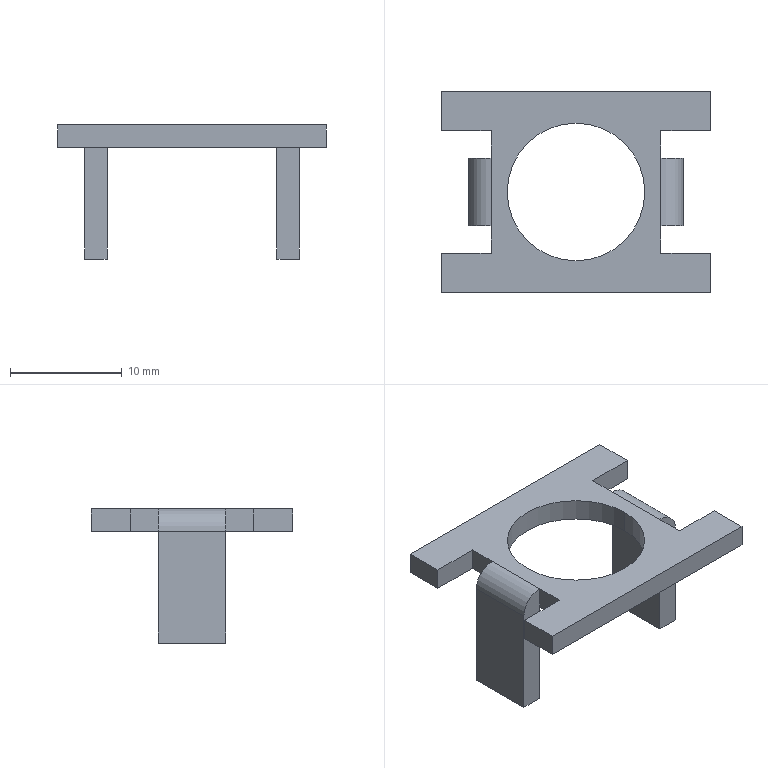Part | STEP file | 0245_Z_016_HCJ8_1 | 1 solid | 30 faces | box 24 x 18 x 12 mm | volume 710.453 mm3 | plane 26 | cylinder 4 | commonest cylinder face diameters 4 x2 12.3 x2